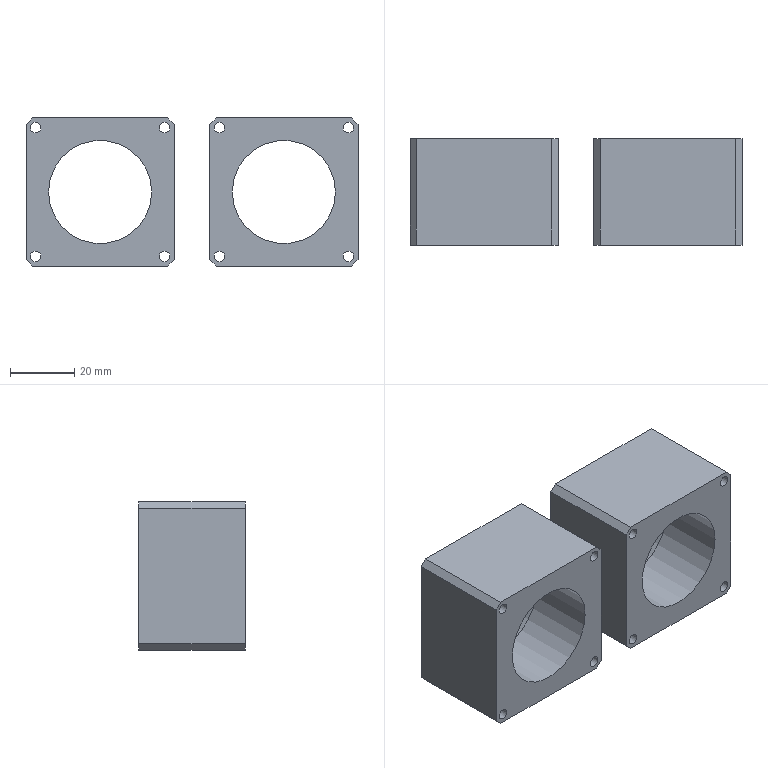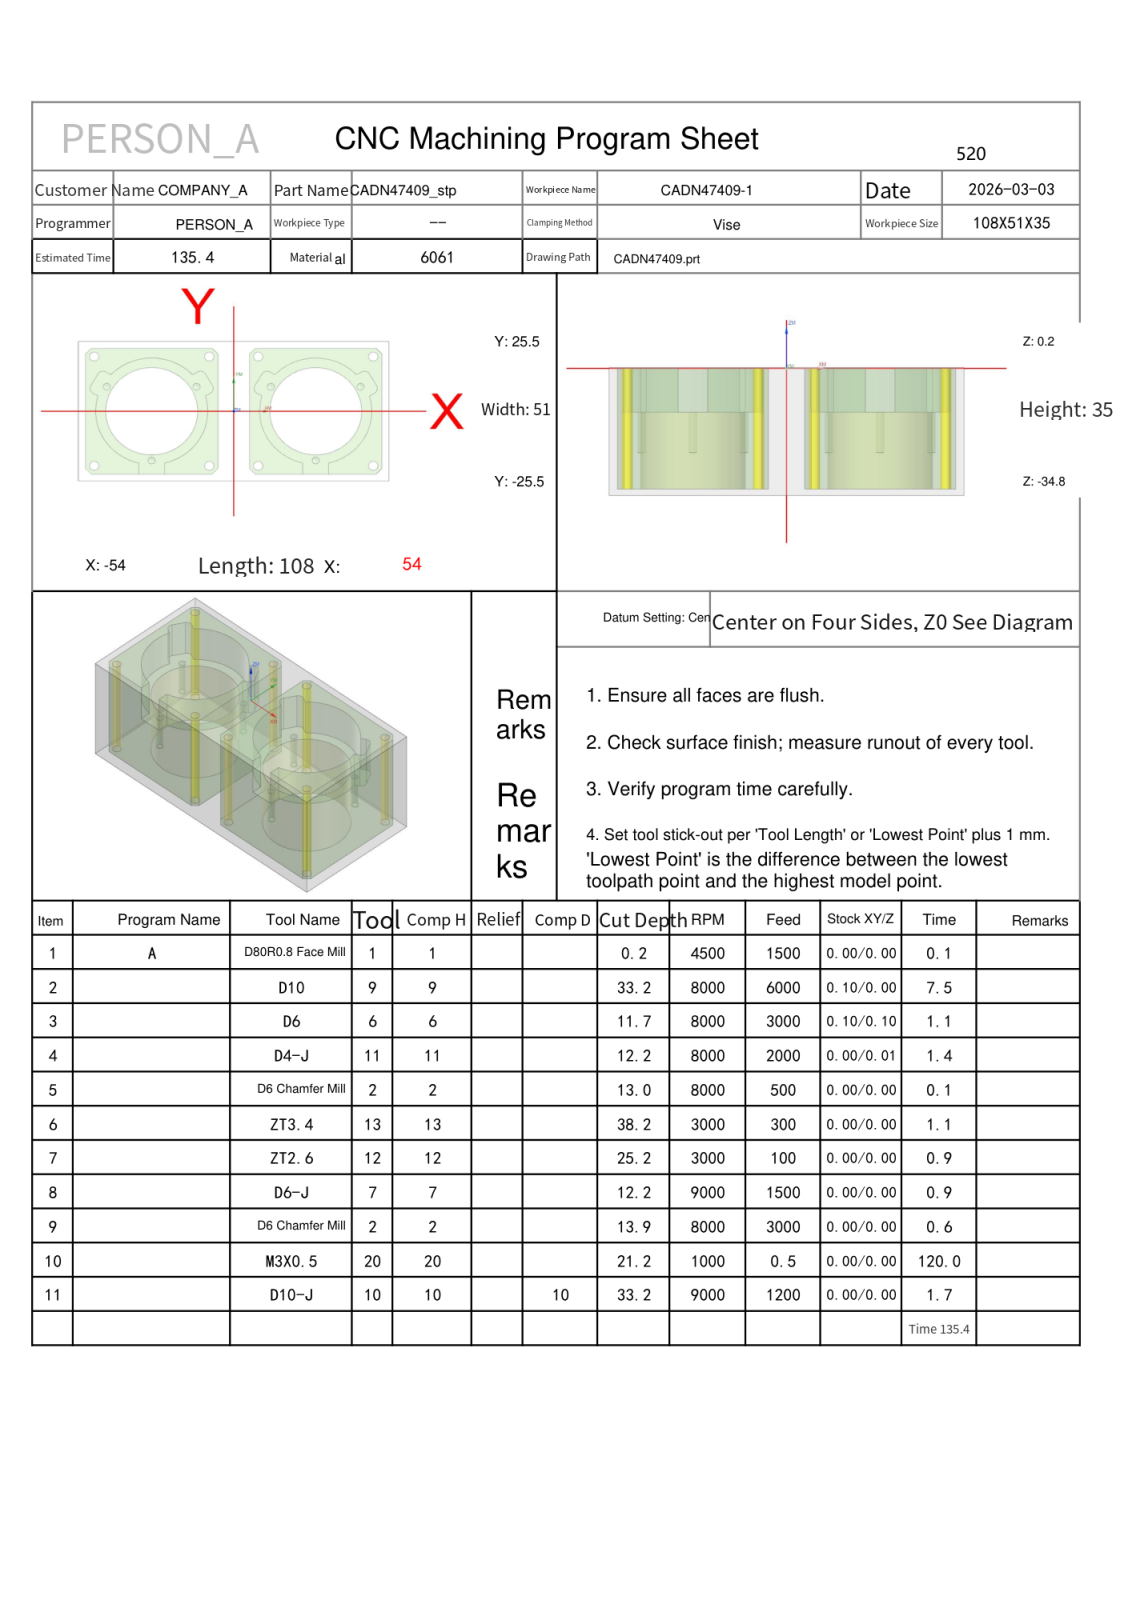NC program | NX | posted by the shop | part box 103 x 33 x 46 mm
Lines 5346 to 6365 of 11287:
N4 T11 M06
(D4-J  D=4. R=0. H=11 ce=0.00 di=0.01)
G00 G90 G54 X-12.329 Y6.374 M03 S8000
G43 H11 Z50.
M08
Z.3
G01 X-12.323 Y6.372 Z.214 F1600.
X-12.304 Y6.366 Z.137
X-12.275 Y6.358 Z.067
X-12.237 Y6.348 Z.004
X-12.192 Y6.338 Z-.052
X-12.14 Y6.328 Z-.101
X-12.084 Y6.32 Z-.143
X-12.025 Y6.314 Z-.18
X-11.964 Y6.311 Z-.211
X-11.903 Y6.313 Z-.237
X-11.843 Y6.32 Z-.257
X-11.786 Y6.333 Z-.274
X-11.733 Y6.354 Z-.286
X-11.686 Y6.383 Z-.294
X-11.646 Y6.421 Z-.298
X-11.615 Y6.469 Z-.3
G02 X-10.818 Y7.322 I1.796 J-.879 F2000.
G01 X-9.071 Y8.331
X-9.063 Y8.335
X-11.563 Y12.665
X-13.318 Y11.652
G02 X-14.318 Y11.384 I-1. J1.732
G01 X-14.455 Y11.389
X-14.497 Y11.375 Z-.301
X-14.523 Y11.328 Z-.303
X-14.534 Y11.251 Z-.306
X-14.532 Y11.148 Z-.311
X-14.517 Y11.022 Z-.317
X-14.49 Y10.876 Z-.324
X-14.453 Y10.713 Z-.332
X-14.351 Y10.359 Z-.35
X-14.276 Y10.129 Z-.361
X-14.14 Y9.757 Z-.381
X-13.883 Y9.172 Z-.415
X-13.585 Y8.608 Z-.45
X-13.246 Y8.069 Z-.485
X-12.868 Y7.555 Z-.519
X-12.614 Y7.252 Z-.538
X-12.453 Y7.072 Z-.55
X-12.197 Y6.808 Z-.568
X-12.075 Y6.694 Z-.576
X-11.962 Y6.598 Z-.582
X-11.861 Y6.522 Z-.588
X-11.773 Y6.469 Z-.593
X-11.701 Y6.441 Z-.597
X-11.648 Y6.44 Z-.599
X-11.615 Y6.469 Z-.6
G02 X-10.818 Y7.322 I1.796 J-.879
G01 X-9.071 Y8.331
X-9.063 Y8.335
X-11.563 Y12.665
X-13.318 Y11.652
G02 X-14.318 Y11.384 I-1. J1.732
G01 X-14.455 Y11.389
X-14.497 Y11.375 Z-.601
X-14.523 Y11.328 Z-.603
X-14.534 Y11.251 Z-.606
X-14.532 Y11.148 Z-.611
X-14.517 Y11.022 Z-.617
X-14.49 Y10.876 Z-.624
X-14.453 Y10.713 Z-.632
X-14.351 Y10.359 Z-.649
X-14.276 Y10.129 Z-.661
X-14.14 Y9.757 Z-.681
X-13.883 Y9.172 Z-.715
X-13.585 Y8.608 Z-.75
X-13.246 Y8.069 Z-.785
X-12.868 Y7.555 Z-.818
X-12.614 Y7.252 Z-.838
X-12.453 Y7.072 Z-.85
X-12.197 Y6.808 Z-.868
X-12.075 Y6.694 Z-.875
X-11.962 Y6.598 Z-.882
X-11.861 Y6.522 Z-.888
X-11.773 Y6.469 Z-.893
X-11.701 Y6.441 Z-.897
X-11.648 Y6.44 Z-.899
X-11.615 Y6.469 Z-.9
G02 X-10.818 Y7.322 I1.796 J-.879
G01 X-9.071 Y8.331
X-9.063 Y8.335
X-11.563 Y12.665
X-13.318 Y11.652
G02 X-14.318 Y11.384 I-1. J1.732
G01 X-14.455 Y11.389
X-14.497 Y11.375
X-14.523 Y11.328 Z-.903
X-14.534 Y11.251 Z-.906
X-14.532 Y11.148 Z-.911
X-14.517 Y11.022 Z-.917
X-14.49 Y10.876 Z-.924
X-14.453 Y10.713 Z-.932
X-14.351 Y10.359 Z-.949
X-14.276 Y10.129 Z-.961
X-14.14 Y9.757 Z-.981
X-13.883 Y9.172 Z-1.015
X-13.585 Y8.608 Z-1.05
X-13.246 Y8.069 Z-1.085
X-12.868 Y7.555 Z-1.118
X-12.614 Y7.252 Z-1.138
X-12.453 Y7.072 Z-1.15
X-12.197 Y6.808 Z-1.167
X-12.075 Y6.694 Z-1.175
X-11.962 Y6.598 Z-1.182
X-11.861 Y6.522 Z-1.188
X-11.773 Y6.469 Z-1.193
X-11.701 Y6.441 Z-1.197
X-11.648 Y6.44 Z-1.199
X-11.615 Y6.469 Z-1.2
G02 X-10.818 Y7.322 I1.796 J-.879
G01 X-9.071 Y8.331
X-9.063 Y8.335
X-11.563 Y12.665
X-13.318 Y11.652
G02 X-14.318 Y11.384 I-1. J1.732
G01 X-14.455 Y11.389
X-14.497 Y11.375
X-14.523 Y11.328 Z-1.202
X-14.534 Y11.251 Z-1.206
X-14.532 Y11.148 Z-1.211
X-14.517 Y11.022 Z-1.217
X-14.49 Y10.876 Z-1.224
X-14.453 Y10.713 Z-1.232
X-14.351 Y10.359 Z-1.249
X-14.276 Y10.129 Z-1.261
X-14.14 Y9.757 Z-1.281
X-13.883 Y9.172 Z-1.314
X-13.585 Y8.608 Z-1.349
X-13.246 Y8.069 Z-1.384
X-12.868 Y7.555 Z-1.418
X-12.614 Y7.252 Z-1.438
X-12.453 Y7.072 Z-1.45
X-12.197 Y6.808 Z-1.467
X-12.075 Y6.694 Z-1.475
X-11.962 Y6.598 Z-1.482
X-11.861 Y6.522 Z-1.488
X-11.773 Y6.469 Z-1.493
X-11.701 Y6.441 Z-1.496
X-11.648 Y6.44 Z-1.499
X-11.615 Y6.469
G02 X-10.818 Y7.322 I1.796 J-.879
G01 X-9.071 Y8.331
X-9.063 Y8.335
X-11.563 Y12.665
X-13.318 Y11.652
G02 X-14.318 Y11.384 I-1. J1.732
G01 X-14.455 Y11.389
X-14.497 Y11.375 Z-1.5
X-14.523 Y11.328 Z-1.502
X-14.534 Y11.251 Z-1.506
X-14.532 Y11.148 Z-1.511
X-14.517 Y11.022 Z-1.517
X-14.49 Y10.876 Z-1.524
X-14.453 Y10.713 Z-1.531
X-14.351 Y10.359 Z-1.549
X-14.276 Y10.129 Z-1.561
X-14.14 Y9.757 Z-1.581
X-13.883 Y9.172 Z-1.614
X-13.585 Y8.608 Z-1.649
X-13.246 Y8.069 Z-1.684
X-12.868 Y7.555 Z-1.718
X-12.614 Y7.252 Z-1.738
X-12.453 Y7.072 Z-1.75
X-12.197 Y6.808 Z-1.767
X-12.075 Y6.694 Z-1.775
X-11.962 Y6.598 Z-1.782
X-11.861 Y6.522 Z-1.788
X-11.773 Y6.469 Z-1.793
X-11.701 Y6.441 Z-1.796
X-11.648 Y6.44 Z-1.798
X-11.615 Y6.469 Z-1.799
G02 X-10.818 Y7.322 I1.796 J-.879
G01 X-9.071 Y8.331
X-9.063 Y8.335
X-11.563 Y12.665
X-13.318 Y11.652
G02 X-14.318 Y11.384 I-1. J1.732
G01 X-14.455 Y11.389
X-14.497 Y11.375 Z-1.8
X-14.523 Y11.328 Z-1.802
X-14.534 Y11.251 Z-1.806
X-14.532 Y11.148 Z-1.811
X-14.517 Y11.022 Z-1.817
X-14.49 Y10.876 Z-1.823
X-14.453 Y10.713 Z-1.831
X-14.351 Y10.359 Z-1.849
X-14.276 Y10.129 Z-1.861
X-14.14 Y9.757 Z-1.88
X-13.883 Y9.172 Z-1.914
X-13.585 Y8.608 Z-1.949
X-13.246 Y8.069 Z-1.984
X-12.868 Y7.555 Z-2.018
X-12.614 Y7.252 Z-2.038
X-12.453 Y7.072 Z-2.049
X-12.197 Y6.808 Z-2.067
X-12.075 Y6.694 Z-2.075
X-11.962 Y6.598 Z-2.082
X-11.861 Y6.522 Z-2.088
X-11.773 Y6.469 Z-2.093
X-11.701 Y6.441 Z-2.096
X-11.648 Y6.44 Z-2.098
X-11.615 Y6.469 Z-2.099
G02 X-10.818 Y7.322 I1.796 J-.879
G01 X-9.071 Y8.331
X-9.063 Y8.335
X-11.563 Y12.665
X-13.318 Y11.652
G02 X-14.318 Y11.384 I-1. J1.732
G01 X-14.455 Y11.389
X-14.497 Y11.375 Z-2.1
X-14.523 Y11.328 Z-2.102
X-14.534 Y11.251 Z-2.106
X-14.532 Y11.148 Z-2.11
X-14.517 Y11.022 Z-2.116
X-14.49 Y10.876 Z-2.123
X-14.453 Y10.713 Z-2.131
X-14.351 Y10.359 Z-2.149
X-14.276 Y10.129 Z-2.161
X-14.14 Y9.757 Z-2.18
X-13.883 Y9.172 Z-2.214
X-13.585 Y8.608 Z-2.249
X-13.246 Y8.069 Z-2.284
X-12.868 Y7.555 Z-2.318
X-12.614 Y7.252 Z-2.338
X-12.453 Y7.072 Z-2.349
X-12.197 Y6.808 Z-2.367
X-12.075 Y6.694 Z-2.375
X-11.962 Y6.598 Z-2.382
X-11.861 Y6.522 Z-2.388
X-11.773 Y6.469 Z-2.392
X-11.701 Y6.441 Z-2.396
X-11.648 Y6.44 Z-2.398
X-11.615 Y6.469 Z-2.399
G02 X-10.818 Y7.322 I1.796 J-.879
G01 X-9.071 Y8.331
X-9.063 Y8.335
X-11.563 Y12.665
X-13.318 Y11.652
G02 X-14.318 Y11.384 I-1. J1.732
G01 X-14.455 Y11.389
X-14.497 Y11.375 Z-2.4
X-14.523 Y11.328 Z-2.402
X-14.534 Y11.251 Z-2.406
X-14.532 Y11.148 Z-2.41
X-14.517 Y11.022 Z-2.416
X-14.49 Y10.876 Z-2.423
X-14.453 Y10.713 Z-2.431
X-14.351 Y10.359 Z-2.449
X-14.276 Y10.129 Z-2.46
X-14.14 Y9.757 Z-2.48
X-13.883 Y9.172 Z-2.514
X-13.585 Y8.608 Z-2.549
X-13.246 Y8.069 Z-2.584
X-12.868 Y7.555 Z-2.618
X-12.614 Y7.252 Z-2.637
X-12.453 Y7.072 Z-2.649
X-12.197 Y6.808 Z-2.667
X-12.075 Y6.694 Z-2.675
X-11.962 Y6.598 Z-2.682
X-11.861 Y6.522 Z-2.688
X-11.773 Y6.469 Z-2.692
X-11.701 Y6.441 Z-2.696
X-11.648 Y6.44 Z-2.698
X-11.615 Y6.469 Z-2.699
G02 X-10.818 Y7.322 I1.796 J-.879
G01 X-9.071 Y8.331
X-9.063 Y8.335
X-11.563 Y12.665
X-13.318 Y11.652
G02 X-14.318 Y11.384 I-1. J1.732
G01 X-14.455 Y11.389
X-14.497 Y11.375 Z-2.7
X-14.523 Y11.328 Z-2.702
X-14.534 Y11.251 Z-2.705
X-14.532 Y11.148 Z-2.71
X-14.517 Y11.022 Z-2.716
X-14.49 Y10.876 Z-2.723
X-14.453 Y10.713 Z-2.731
X-14.351 Y10.359 Z-2.749
X-14.276 Y10.129 Z-2.76
X-14.14 Y9.757 Z-2.78
X-13.883 Y9.172 Z-2.814
X-13.585 Y8.608 Z-2.849
X-13.246 Y8.069 Z-2.884
X-12.868 Y7.555 Z-2.918
X-12.614 Y7.252 Z-2.937
X-12.453 Y7.072 Z-2.949
X-12.197 Y6.808 Z-2.967
X-12.075 Y6.694 Z-2.975
X-11.962 Y6.598 Z-2.981
X-11.861 Y6.522 Z-2.987
X-11.773 Y6.469 Z-2.992
X-11.701 Y6.441 Z-2.996
X-11.648 Y6.44 Z-2.998
X-11.615 Y6.469 Z-2.999
G02 X-10.818 Y7.322 I1.796 J-.879
G01 X-9.071 Y8.331
X-9.063 Y8.335
X-11.563 Y12.665
X-13.318 Y11.652
G02 X-14.318 Y11.384 I-1. J1.732
G01 X-14.455 Y11.389
X-14.497 Y11.375 Z-3.
X-14.523 Y11.328 Z-3.002
X-14.534 Y11.251 Z-3.005
X-14.532 Y11.148 Z-3.01
X-14.517 Y11.022 Z-3.016
X-14.49 Y10.876 Z-3.023
X-14.453 Y10.713 Z-3.031
X-14.351 Y10.359 Z-3.048
X-14.276 Y10.129 Z-3.06
X-14.14 Y9.757 Z-3.08
X-13.883 Y9.172 Z-3.114
X-13.585 Y8.608 Z-3.149
X-13.246 Y8.069 Z-3.184
X-12.868 Y7.555 Z-3.217
X-12.614 Y7.252 Z-3.237
X-12.453 Y7.072 Z-3.249
X-12.197 Y6.808 Z-3.267
X-12.075 Y6.694 Z-3.274
X-11.962 Y6.598 Z-3.281
X-11.861 Y6.522 Z-3.287
X-11.773 Y6.469 Z-3.292
X-11.701 Y6.441 Z-3.296
X-11.648 Y6.44 Z-3.298
X-11.615 Y6.469 Z-3.299
G02 X-10.818 Y7.322 I1.796 J-.879
G01 X-9.071 Y8.331
X-9.063 Y8.335
X-11.563 Y12.665
X-13.318 Y11.652
G02 X-14.318 Y11.384 I-1. J1.732
G01 X-14.455 Y11.389
X-14.497 Y11.375
X-14.523 Y11.328 Z-3.302
X-14.534 Y11.251 Z-3.305
X-14.532 Y11.148 Z-3.31
X-14.517 Y11.022 Z-3.316
X-14.49 Y10.876 Z-3.323
X-14.453 Y10.713 Z-3.331
X-14.351 Y10.359 Z-3.348
X-14.276 Y10.129 Z-3.36
X-14.14 Y9.757 Z-3.38
X-13.883 Y9.172 Z-3.414
X-13.585 Y8.608 Z-3.449
X-13.246 Y8.069 Z-3.484
X-12.868 Y7.555 Z-3.517
X-12.614 Y7.252 Z-3.537
X-12.453 Y7.072 Z-3.549
X-12.197 Y6.808 Z-3.566
X-12.075 Y6.694 Z-3.574
X-11.962 Y6.598 Z-3.581
X-11.861 Y6.522 Z-3.587
X-11.773 Y6.469 Z-3.592
X-11.701 Y6.441 Z-3.596
X-11.648 Y6.44 Z-3.598
X-11.615 Y6.469 Z-3.599
G02 X-10.818 Y7.322 I1.796 J-.879
G01 X-9.071 Y8.331
X-9.063 Y8.335
X-11.563 Y12.665
X-13.318 Y11.652
G02 X-14.318 Y11.384 I-1. J1.732
G01 X-14.455 Y11.389
X-14.497 Y11.375
X-14.523 Y11.328 Z-3.601
X-14.534 Y11.251 Z-3.605
X-14.532 Y11.148 Z-3.61
X-14.517 Y11.022 Z-3.616
X-14.49 Y10.876 Z-3.623
X-14.453 Y10.713 Z-3.631
X-14.351 Y10.359 Z-3.648
X-14.276 Y10.129 Z-3.66
X-14.14 Y9.757 Z-3.68
X-13.883 Y9.172 Z-3.713
X-13.585 Y8.608 Z-3.748
X-13.246 Y8.069 Z-3.783
X-12.868 Y7.555 Z-3.817
X-12.614 Y7.252 Z-3.837
X-12.453 Y7.072 Z-3.849
X-12.197 Y6.808 Z-3.866
X-12.075 Y6.694 Z-3.874
X-11.962 Y6.598 Z-3.881
X-11.861 Y6.522 Z-3.887
X-11.773 Y6.469 Z-3.892
X-11.701 Y6.441 Z-3.895
X-11.648 Y6.44 Z-3.898
X-11.615 Y6.469
G02 X-10.818 Y7.322 I1.796 J-.879
G01 X-9.071 Y8.331
X-9.063 Y8.335
X-11.563 Y12.665
X-13.318 Y11.652
G02 X-14.318 Y11.384 I-1. J1.732
G01 X-14.455 Y11.389
X-14.497 Y11.375 Z-3.899
X-14.523 Y11.328 Z-3.901
X-14.534 Y11.251 Z-3.905
X-14.532 Y11.148 Z-3.91
X-14.517 Y11.022 Z-3.916
X-14.49 Y10.876 Z-3.923
X-14.453 Y10.713 Z-3.93
X-14.351 Y10.359 Z-3.948
X-14.276 Y10.129 Z-3.96
X-14.14 Y9.757 Z-3.98
X-13.883 Y9.172 Z-4.013
X-13.585 Y8.608 Z-4.048
X-13.246 Y8.069 Z-4.083
X-12.868 Y7.555 Z-4.117
X-12.614 Y7.252 Z-4.137
X-12.453 Y7.072 Z-4.149
X-12.197 Y6.808 Z-4.166
X-12.075 Y6.694 Z-4.174
X-11.962 Y6.598 Z-4.181
X-11.861 Y6.522 Z-4.187
X-11.773 Y6.469 Z-4.192
X-11.701 Y6.441 Z-4.195
X-11.648 Y6.44 Z-4.197
X-11.615 Y6.469 Z-4.198
G02 X-10.818 Y7.322 I1.796 J-.879
G01 X-9.071 Y8.331
X-9.063 Y8.335
X-11.563 Y12.665
X-13.318 Y11.652
G02 X-14.318 Y11.384 I-1. J1.732
G01 X-14.455 Y11.389
X-14.497 Y11.375 Z-4.199
X-14.523 Y11.328 Z-4.201
X-14.534 Y11.251 Z-4.205
X-14.532 Y11.148 Z-4.21
X-14.517 Y11.022 Z-4.216
X-14.49 Y10.876 Z-4.222
X-14.453 Y10.713 Z-4.23
X-14.351 Y10.359 Z-4.248
X-14.276 Y10.129 Z-4.26
X-14.14 Y9.757 Z-4.279
X-13.883 Y9.172 Z-4.313
X-13.585 Y8.608 Z-4.348
X-13.246 Y8.069 Z-4.383
X-12.868 Y7.555 Z-4.417
X-12.614 Y7.252 Z-4.437
X-12.453 Y7.072 Z-4.448
X-12.197 Y6.808 Z-4.466
X-12.075 Y6.694 Z-4.474
X-11.962 Y6.598 Z-4.481
X-11.861 Y6.522 Z-4.487
X-11.773 Y6.469 Z-4.492
X-11.701 Y6.441 Z-4.495
X-11.648 Y6.44 Z-4.497
X-11.615 Y6.469 Z-4.498
G02 X-10.818 Y7.322 I1.796 J-.879
G01 X-9.071 Y8.331
X-9.063 Y8.335
X-11.563 Y12.665
X-13.318 Y11.652
G02 X-14.318 Y11.384 I-1. J1.732
G01 X-14.455 Y11.389
X-14.497 Y11.375 Z-4.499
X-14.523 Y11.328 Z-4.501
X-14.534 Y11.251 Z-4.505
X-14.532 Y11.148 Z-4.509
X-14.517 Y11.022 Z-4.515
X-14.49 Y10.876 Z-4.522
X-14.453 Y10.713 Z-4.53
X-14.351 Y10.359 Z-4.548
X-14.276 Y10.129 Z-4.56
X-14.14 Y9.757 Z-4.579
X-13.883 Y9.172 Z-4.613
X-13.585 Y8.608 Z-4.648
X-13.246 Y8.069 Z-4.683
X-12.868 Y7.555 Z-4.717
X-12.614 Y7.252 Z-4.737
X-12.453 Y7.072 Z-4.748
X-12.197 Y6.808 Z-4.766
X-12.075 Y6.694 Z-4.774
X-11.962 Y6.598 Z-4.781
X-11.861 Y6.522 Z-4.787
X-11.773 Y6.469 Z-4.791
X-11.701 Y6.441 Z-4.795
X-11.648 Y6.44 Z-4.797
X-11.615 Y6.469 Z-4.798
G02 X-10.818 Y7.322 I1.796 J-.879
G01 X-9.071 Y8.331
X-9.063 Y8.335
X-11.563 Y12.665
X-13.318 Y11.652
G02 X-14.318 Y11.384 I-1. J1.732
G01 X-14.455 Y11.389
X-14.497 Y11.375 Z-4.799
X-14.523 Y11.328 Z-4.801
X-14.534 Y11.251 Z-4.805
X-14.532 Y11.148 Z-4.809
X-14.517 Y11.022 Z-4.815
X-14.49 Y10.876 Z-4.822
X-14.453 Y10.713 Z-4.83
X-14.351 Y10.359 Z-4.848
X-14.276 Y10.129 Z-4.859
X-14.14 Y9.757 Z-4.879
X-13.883 Y9.172 Z-4.913
X-13.585 Y8.608 Z-4.948
X-13.246 Y8.069 Z-4.983
X-12.868 Y7.555 Z-5.017
X-12.614 Y7.252 Z-5.036
X-12.453 Y7.072 Z-5.048
X-12.197 Y6.808 Z-5.066
X-12.075 Y6.694 Z-5.074
X-11.962 Y6.598 Z-5.081
X-11.861 Y6.522 Z-5.087
X-11.773 Y6.469 Z-5.091
X-11.701 Y6.441 Z-5.095
X-11.648 Y6.44 Z-5.097
X-11.615 Y6.469 Z-5.098
G02 X-10.818 Y7.322 I1.796 J-.879
G01 X-9.071 Y8.331
X-9.063 Y8.335
X-11.563 Y12.665
X-13.318 Y11.652
G02 X-14.318 Y11.384 I-1. J1.732
G01 X-14.455 Y11.389
X-14.497 Y11.375 Z-5.099
X-14.523 Y11.328 Z-5.101
X-14.534 Y11.251 Z-5.104
X-14.532 Y11.148 Z-5.109
X-14.517 Y11.022 Z-5.115
X-14.49 Y10.876 Z-5.122
X-14.453 Y10.713 Z-5.13
X-14.351 Y10.359 Z-5.148
X-14.276 Y10.129 Z-5.159
X-14.14 Y9.757 Z-5.179
X-13.883 Y9.172 Z-5.213
X-13.585 Y8.608 Z-5.248
X-13.246 Y8.069 Z-5.283
X-12.868 Y7.555 Z-5.317
X-12.614 Y7.252 Z-5.336
X-12.453 Y7.072 Z-5.348
X-12.197 Y6.808 Z-5.366
X-12.075 Y6.694 Z-5.374
X-11.962 Y6.598 Z-5.38
X-11.861 Y6.522 Z-5.386
X-11.773 Y6.469 Z-5.391
X-11.701 Y6.441 Z-5.395
X-11.648 Y6.44 Z-5.397
X-11.615 Y6.469 Z-5.398
G02 X-10.818 Y7.322 I1.796 J-.879
G01 X-9.071 Y8.331
X-9.063 Y8.335
X-11.563 Y12.665
X-13.318 Y11.652
G02 X-14.318 Y11.384 I-1. J1.732
G01 X-14.455 Y11.389
X-14.497 Y11.375 Z-5.399
X-14.523 Y11.328 Z-5.401
X-14.534 Y11.251 Z-5.404
X-14.532 Y11.148 Z-5.409
X-14.517 Y11.022 Z-5.415
X-14.49 Y10.876 Z-5.422
X-14.453 Y10.713 Z-5.43
X-14.351 Y10.359 Z-5.447
X-14.276 Y10.129 Z-5.459
X-14.14 Y9.757 Z-5.479
X-13.883 Y9.172 Z-5.513
X-13.585 Y8.608 Z-5.548
X-13.246 Y8.069 Z-5.583
X-12.868 Y7.555 Z-5.616
X-12.614 Y7.252 Z-5.636
X-12.453 Y7.072 Z-5.648
X-12.197 Y6.808 Z-5.666
X-12.075 Y6.694 Z-5.673
X-11.962 Y6.598 Z-5.68
X-11.861 Y6.522 Z-5.686
X-11.773 Y6.469 Z-5.691
X-11.701 Y6.441 Z-5.695
X-11.648 Y6.44 Z-5.697
X-11.615 Y6.469 Z-5.698
G02 X-10.818 Y7.322 I1.796 J-.879
G01 X-9.071 Y8.331
X-9.063 Y8.335
X-11.563 Y12.665
X-13.318 Y11.652
G02 X-14.318 Y11.384 I-1. J1.732
G01 X-14.455 Y11.389
X-14.497 Y11.375
X-14.523 Y11.328 Z-5.701
X-14.534 Y11.251 Z-5.704
X-14.532 Y11.148 Z-5.709
X-14.517 Y11.022 Z-5.715
X-14.49 Y10.876 Z-5.722
X-14.453 Y10.713 Z-5.73
X-14.351 Y10.359 Z-5.747
X-14.276 Y10.129 Z-5.759
X-14.14 Y9.757 Z-5.779
X-13.883 Y9.172 Z-5.813
X-13.585 Y8.608 Z-5.848
X-13.246 Y8.069 Z-5.883
X-12.868 Y7.555 Z-5.916
X-12.614 Y7.252 Z-5.936
X-12.453 Y7.072 Z-5.948
X-12.197 Y6.808 Z-5.965
X-12.075 Y6.694 Z-5.973
X-11.962 Y6.598 Z-5.98
X-11.861 Y6.522 Z-5.986
X-11.773 Y6.469 Z-5.991
X-11.701 Y6.441 Z-5.995
X-11.648 Y6.44 Z-5.997
X-11.615 Y6.469 Z-5.998
G02 X-10.818 Y7.322 I1.796 J-.879
G01 X-9.071 Y8.331
X-9.063 Y8.335
X-11.563 Y12.665
X-13.318 Y11.652
G02 X-14.318 Y11.384 I-1. J1.732
G01 X-14.455 Y11.389
X-14.497 Y11.375
X-14.523 Y11.328 Z-6.
X-14.534 Y11.251 Z-6.004
X-14.532 Y11.148 Z-6.009
X-14.517 Y11.022 Z-6.015
X-14.49 Y10.876 Z-6.022
X-14.453 Y10.713 Z-6.03
X-14.351 Y10.359 Z-6.047
X-14.276 Y10.129 Z-6.059
X-14.14 Y9.757 Z-6.079
X-13.883 Y9.172 Z-6.112
X-13.585 Y8.608 Z-6.147
X-13.246 Y8.069 Z-6.182
X-12.868 Y7.555 Z-6.216
X-12.614 Y7.252 Z-6.236
X-12.453 Y7.072 Z-6.248
X-12.197 Y6.808 Z-6.265
X-12.075 Y6.694 Z-6.273
X-11.962 Y6.598 Z-6.28
X-11.861 Y6.522 Z-6.286
X-11.773 Y6.469 Z-6.291
X-11.701 Y6.441 Z-6.294
X-11.648 Y6.44 Z-6.297
X-11.615 Y6.469
G02 X-10.818 Y7.322 I1.796 J-.879
G01 X-9.071 Y8.331
X-9.063 Y8.335
X-11.563 Y12.665
X-13.318 Y11.652
G02 X-14.318 Y11.384 I-1. J1.732
G01 X-14.455 Y11.389
X-14.497 Y11.375 Z-6.298
X-14.523 Y11.328 Z-6.3
X-14.534 Y11.251 Z-6.304
X-14.532 Y11.148 Z-6.309
X-14.517 Y11.022 Z-6.315
X-14.49 Y10.876 Z-6.322
X-14.453 Y10.713 Z-6.329
X-14.351 Y10.359 Z-6.347
X-14.276 Y10.129 Z-6.359
X-14.14 Y9.757 Z-6.379
X-13.883 Y9.172 Z-6.412
X-13.585 Y8.608 Z-6.447
X-13.246 Y8.069 Z-6.482
X-12.868 Y7.555 Z-6.516
X-12.614 Y7.252 Z-6.536
X-12.453 Y7.072 Z-6.548
X-12.197 Y6.808 Z-6.565
X-12.075 Y6.694 Z-6.573
X-11.962 Y6.598 Z-6.58
X-11.861 Y6.522 Z-6.586
X-11.773 Y6.469 Z-6.591
X-11.701 Y6.441 Z-6.594
X-11.648 Y6.44 Z-6.596
X-11.615 Y6.469 Z-6.597
G02 X-10.818 Y7.322 I1.796 J-.879
G01 X-9.071 Y8.331
X-9.063 Y8.335
X-11.563 Y12.665
X-13.318 Y11.652
G02 X-14.318 Y11.384 I-1. J1.732
G01 X-14.455 Y11.389
X-14.497 Y11.375 Z-6.598
X-14.523 Y11.328 Z-6.6
X-14.534 Y11.251 Z-6.604
X-14.532 Y11.148 Z-6.609
X-14.517 Y11.022 Z-6.615
X-14.49 Y10.876 Z-6.621
X-14.453 Y10.713 Z-6.629
X-14.351 Y10.359 Z-6.647
X-14.276 Y10.129 Z-6.659
X-14.14 Y9.757 Z-6.678
X-13.883 Y9.172 Z-6.712
X-13.585 Y8.608 Z-6.747
X-13.246 Y8.069 Z-6.782
X-12.868 Y7.555 Z-6.816
X-12.614 Y7.252 Z-6.836
X-12.453 Y7.072 Z-6.847
X-12.197 Y6.808 Z-6.865
X-12.075 Y6.694 Z-6.873
X-11.962 Y6.598 Z-6.88
X-11.861 Y6.522 Z-6.886
X-11.773 Y6.469 Z-6.891
X-11.701 Y6.441 Z-6.894
X-11.648 Y6.44 Z-6.896
X-11.615 Y6.469 Z-6.897
G02 X-10.818 Y7.322 I1.796 J-.879
G01 X-9.071 Y8.331
X-9.063 Y8.335
X-11.563 Y12.665
X-13.318 Y11.652
G02 X-14.318 Y11.384 I-1. J1.732
G01 X-14.455 Y11.389
X-14.497 Y11.375 Z-6.898
X-14.523 Y11.328 Z-6.9
X-14.534 Y11.251 Z-6.904
X-14.532 Y11.148 Z-6.908
X-14.517 Y11.022 Z-6.914
X-14.49 Y10.876 Z-6.921
X-14.453 Y10.713 Z-6.929
X-14.351 Y10.359 Z-6.947
X-14.276 Y10.129 Z-6.959
X-14.14 Y9.757 Z-6.978
X-13.883 Y9.172 Z-7.012
X-13.585 Y8.608 Z-7.047
X-13.246 Y8.069 Z-7.082
X-12.868 Y7.555 Z-7.116
X-12.614 Y7.252 Z-7.136
X-12.453 Y7.072 Z-7.147
X-12.197 Y6.808 Z-7.165
X-12.075 Y6.694 Z-7.173
X-11.962 Y6.598 Z-7.18
X-11.861 Y6.522 Z-7.186
X-11.773 Y6.469 Z-7.19
X-11.701 Y6.441 Z-7.194
X-11.648 Y6.44 Z-7.196
X-11.615 Y6.469 Z-7.197
G02 X-10.818 Y7.322 I1.796 J-.879
G01 X-9.071 Y8.331
X-9.063 Y8.335
X-11.563 Y12.665
X-13.318 Y11.652
G02 X-14.318 Y11.384 I-1. J1.732
G01 X-14.455 Y11.389
X-14.497 Y11.375 Z-7.198
X-14.523 Y11.328 Z-7.2
X-14.534 Y11.251 Z-7.204
X-14.532 Y11.148 Z-7.208
X-14.517 Y11.022 Z-7.214
X-14.49 Y10.876 Z-7.221
X-14.453 Y10.713 Z-7.229
X-14.351 Y10.359 Z-7.247
X-14.276 Y10.129 Z-7.258
X-14.14 Y9.757 Z-7.278
X-13.883 Y9.172 Z-7.312
X-13.585 Y8.608 Z-7.347
X-13.246 Y8.069 Z-7.382
X-12.868 Y7.555 Z-7.416
X-12.614 Y7.252 Z-7.435
X-12.453 Y7.072 Z-7.447
X-12.197 Y6.808 Z-7.465
X-12.075 Y6.694 Z-7.473
X-11.962 Y6.598 Z-7.48
X-11.861 Y6.522 Z-7.486
X-11.773 Y6.469 Z-7.49
X-11.701 Y6.441 Z-7.494
X-11.648 Y6.44 Z-7.496
X-11.615 Y6.469 Z-7.497
G02 X-10.818 Y7.322 I1.796 J-.879
G01 X-9.071 Y8.331
X-9.063 Y8.335
X-11.563 Y12.665
X-13.318 Y11.652
G02 X-14.318 Y11.384 I-1. J1.732
G01 X-14.455 Y11.389
X-14.497 Y11.375 Z-7.498
X-14.523 Y11.328 Z-7.5
X-14.534 Y11.251 Z-7.503
X-14.532 Y11.148 Z-7.508
X-14.517 Y11.022 Z-7.514
X-14.49 Y10.876 Z-7.521
X-14.453 Y10.713 Z-7.529
X-14.351 Y10.359 Z-7.547
X-14.276 Y10.129 Z-7.558
X-14.14 Y9.757 Z-7.578
X-13.883 Y9.172 Z-7.612
X-13.585 Y8.608 Z-7.647
X-13.246 Y8.069 Z-7.682
X-12.868 Y7.555 Z-7.716
X-12.614 Y7.252 Z-7.735
X-12.453 Y7.072 Z-7.747
X-12.197 Y6.808 Z-7.765
X-12.075 Y6.694 Z-7.773
X-11.962 Y6.598 Z-7.779
X-11.861 Y6.522 Z-7.785
X-11.773 Y6.469 Z-7.79
X-11.701 Y6.441 Z-7.794
X-11.648 Y6.44 Z-7.796
X-11.615 Y6.469 Z-7.797
G02 X-10.818 Y7.322 I1.796 J-.879
G01 X-9.071 Y8.331
X-9.063 Y8.335
X-11.563 Y12.665
X-13.318 Y11.652
G02 X-14.318 Y11.384 I-1. J1.732
G01 X-14.455 Y11.389
X-14.497 Y11.375 Z-7.798
X-14.523 Y11.328 Z-7.8
X-14.534 Y11.251 Z-7.803
X-14.532 Y11.148 Z-7.808
X-14.517 Y11.022 Z-7.814
X-14.49 Y10.876 Z-7.821
X-14.453 Y10.713 Z-7.829
X-14.351 Y10.359 Z-7.846
X-14.276 Y10.129 Z-7.858
X-14.14 Y9.757 Z-7.878
X-13.883 Y9.172 Z-7.912
X-13.585 Y8.608 Z-7.947
X-13.246 Y8.069 Z-7.982
X-12.868 Y7.555 Z-8.015
X-12.614 Y7.252 Z-8.035
X-12.453 Y7.072 Z-8.047
X-12.197 Y6.808 Z-8.065
X-12.075 Y6.694 Z-8.072
X-11.962 Y6.598 Z-8.079
X-11.861 Y6.522 Z-8.085
X-11.773 Y6.469 Z-8.09
X-11.701 Y6.441 Z-8.094
X-11.648 Y6.44 Z-8.096
X-11.615 Y6.469 Z-8.097
G02 X-10.818 Y7.322 I1.796 J-.879
G01 X-9.071 Y8.331
X-9.063 Y8.335
X-11.563 Y12.665
X-13.318 Y11.652
G02 X-14.318 Y11.384 I-1. J1.732
G01 X-14.455 Y11.389
X-14.497 Y11.375
X-14.523 Y11.328 Z-8.1
X-14.534 Y11.251 Z-8.103
X-14.532 Y11.148 Z-8.108
X-14.517 Y11.022 Z-8.114
X-14.49 Y10.876 Z-8.121
X-14.453 Y10.713 Z-8.129
X-14.351 Y10.359 Z-8.146
X-14.276 Y10.129 Z-8.158
X-14.14 Y9.757 Z-8.178
X-13.883 Y9.172 Z-8.212
X-13.585 Y8.608 Z-8.247
X-13.246 Y8.069 Z-8.282
X-12.868 Y7.555 Z-8.315
X-12.614 Y7.252 Z-8.335
X-12.453 Y7.072 Z-8.347
X-12.197 Y6.808 Z-8.364
X-12.075 Y6.694 Z-8.372
X-11.962 Y6.598 Z-8.379
X-11.861 Y6.522 Z-8.385
X-11.773 Y6.469 Z-8.39
X-11.701 Y6.441 Z-8.394
X-11.648 Y6.44 Z-8.396
X-11.615 Y6.469 Z-8.397
G02 X-10.818 Y7.322 I1.796 J-.879
G01 X-9.071 Y8.331
X-9.063 Y8.335
X-11.563 Y12.665
X-13.318 Y11.652
G02 X-14.318 Y11.384 I-1. J1.732
G01 X-14.455 Y11.389
X-14.497 Y11.375
X-14.523 Y11.328 Z-8.399
X-14.534 Y11.251 Z-8.403
X-14.532 Y11.148 Z-8.408
X-14.517 Y11.022 Z-8.414
X-14.49 Y10.876 Z-8.421
X-14.453 Y10.713 Z-8.429
X-14.351 Y10.359 Z-8.446
X-14.276 Y10.129 Z-8.458
X-14.14 Y9.757 Z-8.478
X-13.883 Y9.172 Z-8.511
X-13.585 Y8.608 Z-8.546
X-13.246 Y8.069 Z-8.581
X-12.868 Y7.555 Z-8.615
X-12.614 Y7.252 Z-8.635
X-12.453 Y7.072 Z-8.647
X-12.197 Y6.808 Z-8.664
X-12.075 Y6.694 Z-8.672
X-11.962 Y6.598 Z-8.679
X-11.861 Y6.522 Z-8.685
X-11.773 Y6.469 Z-8.69
X-11.701 Y6.441 Z-8.693
X-11.648 Y6.44 Z-8.696
X-11.615 Y6.469
G02 X-10.818 Y7.322 I1.796 J-.879
G01 X-9.071 Y8.331
X-9.063 Y8.335
X-11.563 Y12.665
X-13.318 Y11.652
G02 X-14.318 Y11.384 I-1. J1.732
G01 X-14.455 Y11.389
X-14.497 Y11.375 Z-8.697
X-14.523 Y11.328 Z-8.699
X-14.534 Y11.251 Z-8.703
X-14.532 Y11.148 Z-8.708
X-14.517 Y11.022 Z-8.714
X-14.49 Y10.876 Z-8.721
X-14.453 Y10.713 Z-8.728
X-14.351 Y10.359 Z-8.746
X-14.276 Y10.129 Z-8.758
X-14.14 Y9.757 Z-8.778
X-13.883 Y9.172 Z-8.811
X-13.585 Y8.608 Z-8.846
X-13.246 Y8.069 Z-8.881
X-12.868 Y7.555 Z-8.915
X-12.614 Y7.252 Z-8.935
X-12.453 Y7.072 Z-8.947
X-12.197 Y6.808 Z-8.964
X-12.075 Y6.694 Z-8.972
X-11.962 Y6.598 Z-8.979
X-11.861 Y6.522 Z-8.985
X-11.773 Y6.469 Z-8.99
X-11.701 Y6.441 Z-8.993
X-11.648 Y6.44 Z-8.995
X-11.615 Y6.469 Z-8.996
G02 X-10.818 Y7.322 I1.796 J-.879
G01 X-9.071 Y8.331
X-9.063 Y8.335
X-11.563 Y12.665
X-13.318 Y11.652
G02 X-14.318 Y11.384 I-1. J1.732
G01 X-14.455 Y11.389
X-14.497 Y11.375 Z-8.997
X-14.523 Y11.328 Z-8.999
X-14.534 Y11.251 Z-9.003
X-14.532 Y11.148 Z-9.008
X-14.517 Y11.022 Z-9.014
X-14.49 Y10.876 Z-9.02
X-14.453 Y10.713 Z-9.028
X-14.351 Y10.359 Z-9.046
X-14.276 Y10.129 Z-9.058
X-14.14 Y9.757 Z-9.077
X-13.883 Y9.172 Z-9.111
X-13.585 Y8.608 Z-9.146
X-13.246 Y8.069 Z-9.181
X-12.868 Y7.555 Z-9.215
X-12.614 Y7.252 Z-9.235
X-12.453 Y7.072 Z-9.246
X-12.197 Y6.808 Z-9.264
X-12.075 Y6.694 Z-9.272
X-11.962 Y6.598 Z-9.279
X-11.861 Y6.522 Z-9.285
X-11.773 Y6.469 Z-9.29
X-11.701 Y6.441 Z-9.293
X-11.648 Y6.44 Z-9.295
X-11.615 Y6.469 Z-9.296
G02 X-10.818 Y7.322 I1.796 J-.879
G01 X-9.071 Y8.331
X-9.063 Y8.335
X-11.563 Y12.665
X-13.318 Y11.652
G02 X-14.318 Y11.384 I-1. J1.732
G01 X-14.455 Y11.389
X-14.497 Y11.375 Z-9.297
X-14.523 Y11.328 Z-9.299
X-14.534 Y11.251 Z-9.303
X-14.532 Y11.148 Z-9.307
X-14.517 Y11.022 Z-9.313
X-14.49 Y10.876 Z-9.32
X-14.453 Y10.713 Z-9.328
X-14.351 Y10.359 Z-9.346
X-14.276 Y10.129 Z-9.358
X-14.14 Y9.757 Z-9.377
X-13.883 Y9.172 Z-9.411
X-13.585 Y8.608 Z-9.446
X-13.246 Y8.069 Z-9.481
X-12.868 Y7.555 Z-9.515
X-12.614 Y7.252 Z-9.535
X-12.453 Y7.072 Z-9.546
X-12.197 Y6.808 Z-9.564
X-12.075 Y6.694 Z-9.572
X-11.962 Y6.598 Z-9.579
X-11.861 Y6.522 Z-9.585
X-11.773 Y6.469 Z-9.589
X-11.701 Y6.441 Z-9.593
X-11.648 Y6.44 Z-9.595
X-11.615 Y6.469 Z-9.596
G02 X-10.818 Y7.322 I1.796 J-.879
G01 X-9.071 Y8.331
X-9.063 Y8.335
X-11.563 Y12.665
X-13.318 Y11.652
G02 X-14.318 Y11.384 I-1. J1.732
G01 X-14.455 Y11.389
X-14.497 Y11.375 Z-9.597
X-14.523 Y11.328 Z-9.599
X-14.534 Y11.251 Z-9.603
X-14.532 Y11.148 Z-9.607
X-14.517 Y11.022 Z-9.613
X-14.49 Y10.876 Z-9.62
X-14.453 Y10.713 Z-9.628
X-14.351 Y10.359 Z-9.646
X-14.276 Y10.129 Z-9.657
X-14.14 Y9.757 Z-9.677
X-13.883 Y9.172 Z-9.711
X-13.585 Y8.608 Z-9.746
X-13.246 Y8.069 Z-9.781
X-12.868 Y7.555 Z-9.815
X-12.614 Y7.252 Z-9.834
X-12.453 Y7.072 Z-9.846
X-12.197 Y6.808 Z-9.864
X-12.075 Y6.694 Z-9.872
X-11.962 Y6.598 Z-9.879
X-11.861 Y6.522 Z-9.885
X-11.773 Y6.469 Z-9.889
X-11.701 Y6.441 Z-9.893
X-11.648 Y6.44 Z-9.895
X-11.615 Y6.469 Z-9.896
G02 X-10.818 Y7.322 I1.796 J-.879
G01 X-9.071 Y8.331
X-9.063 Y8.335
X-11.563 Y12.665
X-13.318 Y11.652
G02 X-14.318 Y11.384 I-1. J1.732